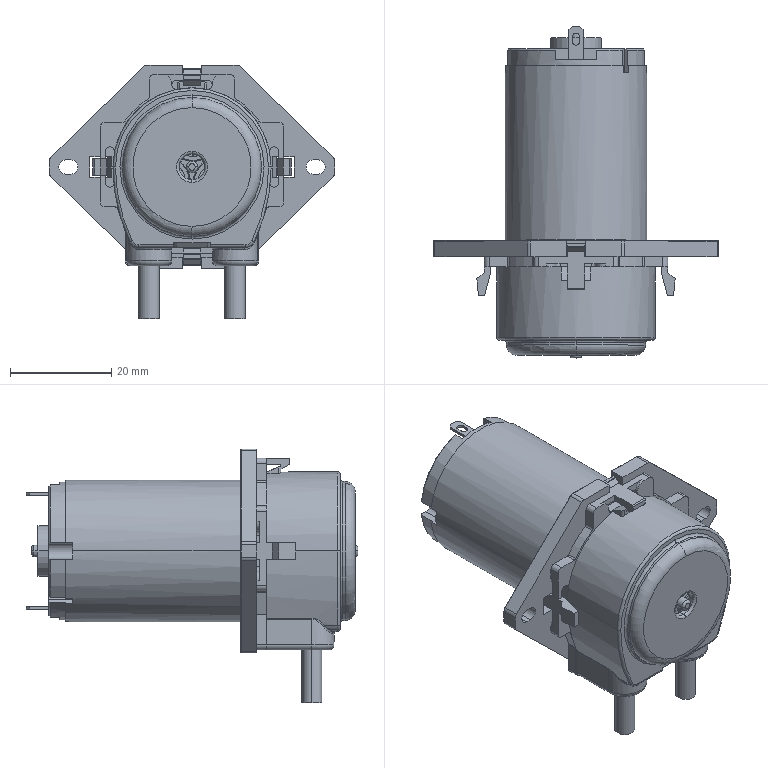Part | SolidWorks | 12 solids | 887 faces | box 56.3 x 65.53 x 50.125 mm | volume 38385 mm3 | plane 425 | cylinder 319 | torus 77 | cone 42 | sphere 16 | spline 8 | commonest cylinder face diameters 0.2 x28 2 x26 2.515 x26 0.5 x24 1.799 x24 1 x20